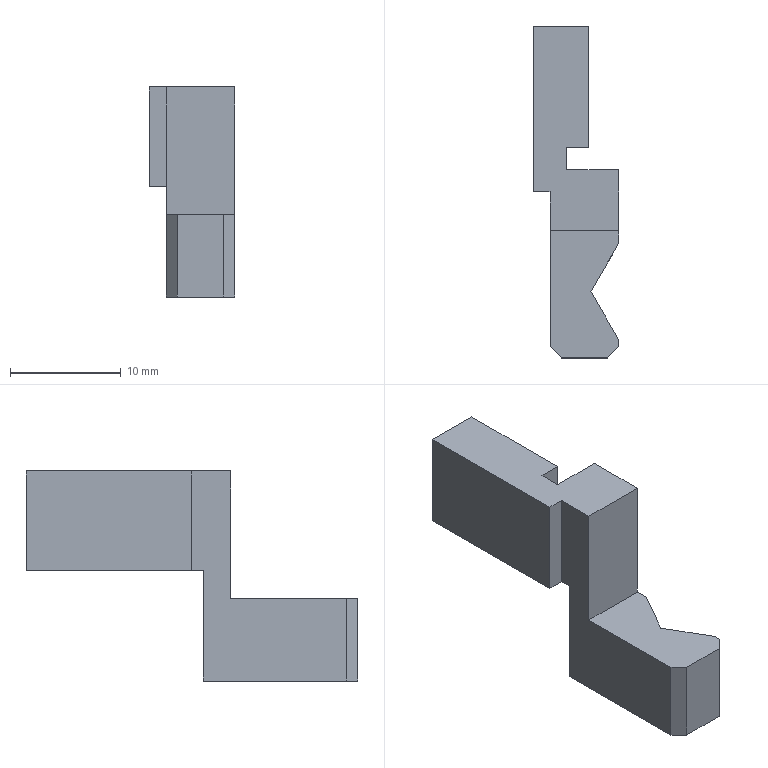Part | STEP file | 2012-06-08-016 | 1 solid | 25 faces | box 7.7 x 30 x 19 mm | volume 1396 mm3 | plane 25